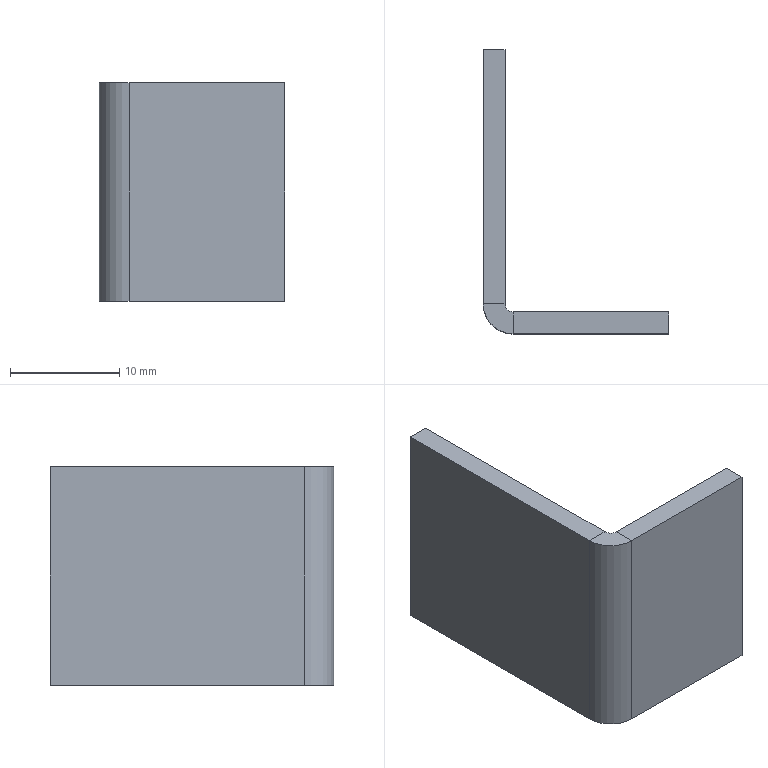Part | SolidWorks | features FlatPattern 1, SMBaseFlange 1, SheetMetal 1 | 1 solid | 14 faces | box 17 x 26 x 20 mm | volume 1610 mm3 | plane 12 | cylinder 2 | commonest cylinder face diameters 1.473 x1 5.473 x1
STEP:
#1=CARTESIAN_POINT('',(0.7366,0.,10.));
#2=VERTEX_POINT('',#1);
#3=CARTESIAN_POINT('',(0.7366,-2.,10.));
#4=VERTEX_POINT('',#3);
#5=CARTESIAN_POINT('',(0.7366,0.,10.));
#6=DIRECTION('',(0.,-1.,0.));
#7=VECTOR('',#6,1000.);
#8=LINE('',#5,#7);
#9=EDGE_CURVE('',#2,#4,#8,.T.);
#10=ORIENTED_EDGE('',*,*,#9,.F.);
#11=CARTESIAN_POINT('',(0.,0.7366,10.));
#12=VERTEX_POINT('',#11);
#13=CARTESIAN_POINT('',(0.7366,0.7366,10.));
#14=DIRECTION('',(0.,0.,1.));
#15=DIRECTION('',(-1.,0.,0.));
#16=AXIS2_PLACEMENT_3D('',#13,#14,#15);
#17=CIRCLE('',#16,0.7366);
#18=EDGE_CURVE('',#12,#2,#17,.T.);
#19=ORIENTED_EDGE('',*,*,#18,.F.);
#20=CARTESIAN_POINT('',(-2.,0.7366,10.));
#21=VERTEX_POINT('',#20);
#22=CARTESIAN_POINT('',(-2.,0.7366,10.));
#23=DIRECTION('',(1.,0.,0.));
#24=VECTOR('',#23,1000.);
#25=LINE('',#22,#24);
#26=EDGE_CURVE('',#21,#12,#25,.T.);
#27=ORIENTED_EDGE('',*,*,#26,.F.);
#28=CARTESIAN_POINT('',(0.7366,0.7366,10.));
#29=DIRECTION('',(0.,0.,1.));
#30=DIRECTION('',(1.,0.,0.));
#31=AXIS2_PLACEMENT_3D('',#28,#29,#30);
#32=CIRCLE('',#31,2.737);
#33=EDGE_CURVE('',#21,#4,#32,.T.);
#34=ORIENTED_EDGE('',*,*,#33,.T.);
#35=EDGE_LOOP('',(#10,#19,#27,#34));
#36=FACE_OUTER_BOUND('',#35,.T.);
#37=CARTESIAN_POINT('',(0.7366,0.,10.));
#38=DIRECTION('',(0.,0.,1.));
#39=DIRECTION('',(1.,0.,0.));
#40=AXIS2_PLACEMENT_3D('',#37,#38,#39);
#41=PLANE('',#40);
#42=ADVANCED_FACE('',(#36),#41,.T.);
#43=CARTESIAN_POINT('',(15.,0.,10.));
#44=VERTEX_POINT('',#43);
#45=CARTESIAN_POINT('',(0.,0.,10.));
#46=DIRECTION('',(1.,0.,0.));
#47=VECTOR('',#46,1000.);
#48=LINE('',#45,#47);
#49=EDGE_CURVE('',#2,#44,#48,.T.);
#50=ORIENTED_EDGE('',*,*,#49,.F.);
#51=ORIENTED_EDGE('',*,*,#9,.T.);
#52=CARTESIAN_POINT('',(15.,-2.,10.));
#53=VERTEX_POINT('',#52);
#54=CARTESIAN_POINT('',(0.,-2.,10.));
#55=DIRECTION('',(1.,0.,0.));
#56=VECTOR('',#55,1000.);
#57=LINE('',#54,#56);
#58=EDGE_CURVE('',#4,#53,#57,.T.);
#59=ORIENTED_EDGE('',*,*,#58,.T.);
#60=CARTESIAN_POINT('',(15.,0.,10.));
#61=DIRECTION('',(0.,-1.,0.));
#62=VECTOR('',#61,1000.);
#63=LINE('',#60,#62);
#64=EDGE_CURVE('',#44,#53,#63,.T.);
#65=ORIENTED_EDGE('',*,*,#64,.F.);
#66=EDGE_LOOP('',(#50,#51,#59,#65));
#67=FACE_OUTER_BOUND('',#66,.T.);
#68=CARTESIAN_POINT('',(-2.,0.7366,10.));
#69=DIRECTION('',(0.,0.,1.));
#70=DIRECTION('',(1.,0.,0.));
#71=AXIS2_PLACEMENT_3D('',#68,#69,#70);
#72=PLANE('',#71);
#73=ADVANCED_FACE('',(#67),#72,.T.);
#74=CARTESIAN_POINT('',(0.,0.7366,-10.));
#75=VERTEX_POINT('',#74);
#76=CARTESIAN_POINT('',(-2.,0.7366,-10.));
#77=VERTEX_POINT('',#76);
#78=CARTESIAN_POINT('',(0.,0.7366,-10.));
#79=DIRECTION('',(-1.,0.,0.));
#80=VECTOR('',#79,1000.);
#81=LINE('',#78,#80);
#82=EDGE_CURVE('',#75,#77,#81,.T.);
#83=ORIENTED_EDGE('',*,*,#82,.F.);
#84=CARTESIAN_POINT('',(0.7366,0.,-10.));
#85=VERTEX_POINT('',#84);
#86=CARTESIAN_POINT('',(0.7366,0.7366,-10.));
#87=DIRECTION('',(0.,0.,1.));
#88=DIRECTION('',(-1.,0.,0.));
#89=AXIS2_PLACEMENT_3D('',#86,#87,#88);
#90=CIRCLE('',#89,0.7366);
#91=EDGE_CURVE('',#75,#85,#90,.T.);
#92=ORIENTED_EDGE('',*,*,#91,.T.);
#93=CARTESIAN_POINT('',(0.7366,-2.,-10.));
#94=VERTEX_POINT('',#93);
#95=CARTESIAN_POINT('',(0.7366,-2.,-10.));
#96=DIRECTION('',(0.,1.,0.));
#97=VECTOR('',#96,1000.);
#98=LINE('',#95,#97);
#99=EDGE_CURVE('',#94,#85,#98,.T.);
#100=ORIENTED_EDGE('',*,*,#99,.F.);
#101=CARTESIAN_POINT('',(0.7366,0.7366,-10.));
#102=DIRECTION('',(0.,0.,1.));
#103=DIRECTION('',(1.,0.,0.));
#104=AXIS2_PLACEMENT_3D('',#101,#102,#103);
#105=CIRCLE('',#104,2.737);
#106=EDGE_CURVE('',#77,#94,#105,.T.);
#107=ORIENTED_EDGE('',*,*,#106,.F.);
#108=EDGE_LOOP('',(#83,#92,#100,#107));
#109=FACE_OUTER_BOUND('',#108,.T.);
#110=CARTESIAN_POINT('',(0.,0.7366,-10.));
#111=DIRECTION('',(0.,0.,-1.));
#112=DIRECTION('',(-1.,0.,0.));
#113=AXIS2_PLACEMENT_3D('',#110,#111,#112);
#114=PLANE('',#113);
#115=ADVANCED_FACE('',(#109),#114,.T.);
#116=CARTESIAN_POINT('',(0.,24.,-10.));
#117=VERTEX_POINT('',#116);
#118=CARTESIAN_POINT('',(0.,0.,-10.));
#119=DIRECTION('',(0.,-1.,0.));
#120=VECTOR('',#119,1000.);
#121=LINE('',#118,#120);
#122=EDGE_CURVE('',#117,#75,#121,.T.);
#123=ORIENTED_EDGE('',*,*,#122,.T.);
#124=ORIENTED_EDGE('',*,*,#82,.T.);
#125=CARTESIAN_POINT('',(-2.,24.,-10.));
#126=VERTEX_POINT('',#125);
#127=CARTESIAN_POINT('',(-2.,0.,-10.));
#128=DIRECTION('',(0.,-1.,0.));
#129=VECTOR('',#128,1000.);
#130=LINE('',#127,#129);
#131=EDGE_CURVE('',#126,#77,#130,.T.);
#132=ORIENTED_EDGE('',*,*,#131,.F.);
#133=CARTESIAN_POINT('',(-2.,24.,-10.));
#134=DIRECTION('',(1.,0.,0.));
#135=VECTOR('',#134,1000.);
#136=LINE('',#133,#135);
#137=EDGE_CURVE('',#126,#117,#136,.T.);
#138=ORIENTED_EDGE('',*,*,#137,.T.);
#139=EDGE_LOOP('',(#123,#124,#132,#138));
#140=FACE_OUTER_BOUND('',#139,.T.);
#141=CARTESIAN_POINT('',(0.7366,-2.,-10.));
#142=DIRECTION('',(0.,0.,-1.));
#143=DIRECTION('',(-1.,0.,0.));
#144=AXIS2_PLACEMENT_3D('',#141,#142,#143);
#145=PLANE('',#144);
#146=ADVANCED_FACE('',(#140),#145,.T.);
#147=CARTESIAN_POINT('',(15.,-2.,-10.));
#148=VERTEX_POINT('',#147);
#149=CARTESIAN_POINT('',(0.,-2.,-10.));
#150=DIRECTION('',(1.,0.,0.));
#151=VECTOR('',#150,1000.);
#152=LINE('',#149,#151);
#153=EDGE_CURVE('',#94,#148,#152,.T.);
#154=ORIENTED_EDGE('',*,*,#153,.T.);
#155=CARTESIAN_POINT('',(15.,-2.,10.));
#156=DIRECTION('',(0.,0.,-1.));
#157=VECTOR('',#156,1000.);
#158=LINE('',#155,#157);
#159=EDGE_CURVE('',#53,#148,#158,.T.);
#160=ORIENTED_EDGE('',*,*,#159,.F.);
#161=ORIENTED_EDGE('',*,*,#58,.F.);
#162=CARTESIAN_POINT('',(0.7366,-2.,10.));
#163=DIRECTION('',(0.,0.,-1.));
#164=VECTOR('',#163,1000.);
#165=LINE('',#162,#164);
#166=EDGE_CURVE('',#4,#94,#165,.T.);
#167=ORIENTED_EDGE('',*,*,#166,.T.);
#168=EDGE_LOOP('',(#154,#160,#161,#167));
#169=FACE_OUTER_BOUND('',#168,.T.);
#170=CARTESIAN_POINT('',(0.,-2.,10.));
#171=DIRECTION('',(0.,1.,0.));
#172=DIRECTION('',(0.,0.,1.));
#173=AXIS2_PLACEMENT_3D('',#170,#171,#172);
#174=PLANE('',#173);
#175=ADVANCED_FACE('',(#169),#174,.F.);
#176=CARTESIAN_POINT('',(15.,0.,-10.));
#177=VERTEX_POINT('',#176);
#178=CARTESIAN_POINT('',(15.,0.,-10.));
#179=DIRECTION('',(0.,-1.,0.));
#180=VECTOR('',#179,1000.);
#181=LINE('',#178,#180);
#182=EDGE_CURVE('',#177,#148,#181,.T.);
#183=ORIENTED_EDGE('',*,*,#182,.F.);
#184=CARTESIAN_POINT('',(15.,0.,10.));
#185=DIRECTION('',(0.,0.,-1.));
#186=VECTOR('',#185,1000.);
#187=LINE('',#184,#186);
#188=EDGE_CURVE('',#44,#177,#187,.T.);
#189=ORIENTED_EDGE('',*,*,#188,.F.);
#190=ORIENTED_EDGE('',*,*,#64,.T.);
#191=ORIENTED_EDGE('',*,*,#159,.T.);
#192=EDGE_LOOP('',(#183,#189,#190,#191));
#193=FACE_OUTER_BOUND('',#192,.T.);
#194=CARTESIAN_POINT('',(15.,0.,10.));
#195=DIRECTION('',(1.,0.,0.));
#196=DIRECTION('',(0.,0.,-1.));
#197=AXIS2_PLACEMENT_3D('',#194,#195,#196);
#198=PLANE('',#197);
#199=ADVANCED_FACE('',(#193),#198,.T.);
#200=CARTESIAN_POINT('',(0.,0.,-10.));
#201=DIRECTION('',(1.,0.,0.));
#202=VECTOR('',#201,1000.);
#203=LINE('',#200,#202);
#204=EDGE_CURVE('',#85,#177,#203,.T.);
#205=ORIENTED_EDGE('',*,*,#204,.F.);
#206=CARTESIAN_POINT('',(0.7366,0.,10.));
#207=DIRECTION('',(0.,0.,-1.));
#208=VECTOR('',#207,1000.);
#209=LINE('',#206,#208);
#210=EDGE_CURVE('',#2,#85,#209,.T.);
#211=ORIENTED_EDGE('',*,*,#210,.F.);
#212=ORIENTED_EDGE('',*,*,#49,.T.);
#213=ORIENTED_EDGE('',*,*,#188,.T.);
#214=EDGE_LOOP('',(#205,#211,#212,#213));
#215=FACE_OUTER_BOUND('',#214,.T.);
#216=CARTESIAN_POINT('',(0.,0.,10.));
#217=DIRECTION('',(0.,1.,0.));
#218=DIRECTION('',(0.,0.,1.));
#219=AXIS2_PLACEMENT_3D('',#216,#217,#218);
#220=PLANE('',#219);
#221=ADVANCED_FACE('',(#215),#220,.T.);
#222=ORIENTED_EDGE('',*,*,#91,.F.);
#223=CARTESIAN_POINT('',(0.,0.7366,10.));
#224=DIRECTION('',(0.,0.,-1.));
#225=VECTOR('',#224,1000.);
#226=LINE('',#223,#225);
#227=EDGE_CURVE('',#12,#75,#226,.T.);
#228=ORIENTED_EDGE('',*,*,#227,.F.);
#229=ORIENTED_EDGE('',*,*,#18,.T.);
#230=ORIENTED_EDGE('',*,*,#210,.T.);
#231=EDGE_LOOP('',(#222,#228,#229,#230));
#232=FACE_OUTER_BOUND('',#231,.T.);
#233=CARTESIAN_POINT('',(0.7366,0.7366,10.));
#234=DIRECTION('',(0.,0.,-1.));
#235=DIRECTION('',(-1.,0.,0.));
#236=AXIS2_PLACEMENT_3D('',#233,#234,#235);
#237=CYLINDRICAL_SURFACE('',#236,0.7366);
#238=ADVANCED_FACE('',(#232),#237,.F.);
#239=ORIENTED_EDGE('',*,*,#122,.F.);
#240=CARTESIAN_POINT('',(0.,24.,10.));
#241=VERTEX_POINT('',#240);
#242=CARTESIAN_POINT('',(0.,24.,10.));
#243=DIRECTION('',(0.,0.,-1.));
#244=VECTOR('',#243,1000.);
#245=LINE('',#242,#244);
#246=EDGE_CURVE('',#241,#117,#245,.T.);
#247=ORIENTED_EDGE('',*,*,#246,.F.);
#248=CARTESIAN_POINT('',(0.,0.,10.));
#249=DIRECTION('',(0.,-1.,0.));
#250=VECTOR('',#249,1000.);
#251=LINE('',#248,#250);
#252=EDGE_CURVE('',#241,#12,#251,.T.);
#253=ORIENTED_EDGE('',*,*,#252,.T.);
#254=ORIENTED_EDGE('',*,*,#227,.T.);
#255=EDGE_LOOP('',(#239,#247,#253,#254));
#256=FACE_OUTER_BOUND('',#255,.T.);
#257=CARTESIAN_POINT('',(0.,0.,10.));
#258=DIRECTION('',(1.,0.,0.));
#259=DIRECTION('',(0.,0.,-1.));
#260=AXIS2_PLACEMENT_3D('',#257,#258,#259);
#261=PLANE('',#260);
#262=ADVANCED_FACE('',(#256),#261,.T.);
#263=ORIENTED_EDGE('',*,*,#137,.F.);
#264=CARTESIAN_POINT('',(-2.,24.,10.));
#265=VERTEX_POINT('',#264);
#266=CARTESIAN_POINT('',(-2.,24.,10.));
#267=DIRECTION('',(0.,0.,-1.));
#268=VECTOR('',#267,1000.);
#269=LINE('',#266,#268);
#270=EDGE_CURVE('',#265,#126,#269,.T.);
#271=ORIENTED_EDGE('',*,*,#270,.F.);
#272=CARTESIAN_POINT('',(-2.,24.,10.));
#273=DIRECTION('',(1.,0.,0.));
#274=VECTOR('',#273,1000.);
#275=LINE('',#272,#274);
#276=EDGE_CURVE('',#265,#241,#275,.T.);
#277=ORIENTED_EDGE('',*,*,#276,.T.);
#278=ORIENTED_EDGE('',*,*,#246,.T.);
#279=EDGE_LOOP('',(#263,#271,#277,#278));
#280=FACE_OUTER_BOUND('',#279,.T.);
#281=CARTESIAN_POINT('',(-2.,24.,10.));
#282=DIRECTION('',(0.,1.,0.));
#283=DIRECTION('',(0.,0.,1.));
#284=AXIS2_PLACEMENT_3D('',#281,#282,#283);
#285=PLANE('',#284);
#286=ADVANCED_FACE('',(#280),#285,.T.);
#287=ORIENTED_EDGE('',*,*,#131,.T.);
#288=CARTESIAN_POINT('',(-2.,0.7366,10.));
#289=DIRECTION('',(0.,0.,-1.));
#290=VECTOR('',#289,1000.);
#291=LINE('',#288,#290);
#292=EDGE_CURVE('',#21,#77,#291,.T.);
#293=ORIENTED_EDGE('',*,*,#292,.F.);
#294=CARTESIAN_POINT('',(-2.,0.,10.));
#295=DIRECTION('',(0.,-1.,0.));
#296=VECTOR('',#295,1000.);
#297=LINE('',#294,#296);
#298=EDGE_CURVE('',#265,#21,#297,.T.);
#299=ORIENTED_EDGE('',*,*,#298,.F.);
#300=ORIENTED_EDGE('',*,*,#270,.T.);
#301=EDGE_LOOP('',(#287,#293,#299,#300));
#302=FACE_OUTER_BOUND('',#301,.T.);
#303=CARTESIAN_POINT('',(-2.,0.,10.));
#304=DIRECTION('',(1.,0.,0.));
#305=DIRECTION('',(0.,0.,-1.));
#306=AXIS2_PLACEMENT_3D('',#303,#304,#305);
#307=PLANE('',#306);
#308=ADVANCED_FACE('',(#302),#307,.F.);
#309=ORIENTED_EDGE('',*,*,#106,.T.);
#310=ORIENTED_EDGE('',*,*,#166,.F.);
#311=ORIENTED_EDGE('',*,*,#33,.F.);
#312=ORIENTED_EDGE('',*,*,#292,.T.);
#313=EDGE_LOOP('',(#309,#310,#311,#312));
#314=FACE_OUTER_BOUND('',#313,.T.);
#315=CARTESIAN_POINT('',(0.7366,0.7366,10.));
#316=DIRECTION('',(0.,0.,-1.));
#317=DIRECTION('',(-1.,0.,0.));
#318=AXIS2_PLACEMENT_3D('',#315,#316,#317);
#319=CYLINDRICAL_SURFACE('',#318,2.737);
#320=ADVANCED_FACE('',(#314),#319,.T.);
#321=ORIENTED_EDGE('',*,*,#298,.T.);
#322=ORIENTED_EDGE('',*,*,#26,.T.);
#323=ORIENTED_EDGE('',*,*,#252,.F.);
#324=ORIENTED_EDGE('',*,*,#276,.F.);
#325=EDGE_LOOP('',(#321,#322,#323,#324));
#326=FACE_OUTER_BOUND('',#325,.T.);
#327=CARTESIAN_POINT('',(0.7366,0.7366,10.));
#328=DIRECTION('',(0.,0.,-1.));
#329=DIRECTION('',(-1.,0.,0.));
#330=AXIS2_PLACEMENT_3D('',#327,#328,#329);
#331=PLANE('',#330);
#332=ADVANCED_FACE('',(#326),#331,.F.);
#333=ORIENTED_EDGE('',*,*,#153,.F.);
#334=ORIENTED_EDGE('',*,*,#99,.T.);
#335=ORIENTED_EDGE('',*,*,#204,.T.);
#336=ORIENTED_EDGE('',*,*,#182,.T.);
#337=EDGE_LOOP('',(#333,#334,#335,#336));
#338=FACE_OUTER_BOUND('',#337,.T.);
#339=CARTESIAN_POINT('',(0.7366,0.7366,-10.));
#340=DIRECTION('',(0.,0.,-1.));
#341=DIRECTION('',(-1.,0.,0.));
#342=AXIS2_PLACEMENT_3D('',#339,#340,#341);
#343=PLANE('',#342);
#344=ADVANCED_FACE('',(#338),#343,.T.);
#345=CLOSED_SHELL('',(#42,#73,#115,#146,#175,#199,#221,#238,#262,#286,#308,#320,#332,#344));
#346=MANIFOLD_SOLID_BREP('',#345);
#347=CARTESIAN_POINT('',(0.,0.,0.));
#348=DIRECTION('',(0.,0.,1.));
#349=DIRECTION('',(1.,0.,0.));
#350=AXIS2_PLACEMENT_3D('',#347,#348,#349);
#351=(LENGTH_UNIT()NAMED_UNIT(*)SI_UNIT(.MILLI.,.METRE.));
#352=UNCERTAINTY_MEASURE_WITH_UNIT(LENGTH_MEASURE(0.00001),#351,'','');
#353=(NAMED_UNIT(*)PLANE_ANGLE_UNIT()SI_UNIT($,.RADIAN.));
#354=(NAMED_UNIT(*)SI_UNIT($,.STERADIAN.)SOLID_ANGLE_UNIT());
#355=(GEOMETRIC_REPRESENTATION_CONTEXT(3)GLOBAL_UNCERTAINTY_ASSIGNED_CONTEXT((#352))GLOBAL_UNIT_ASSIGNED_CONTEXT((#351,#353,#354))REPRESENTATION_CONTEXT('',''));
#356=ADVANCED_BREP_SHAPE_REPRESENTATION('',(#346,#350),#355);